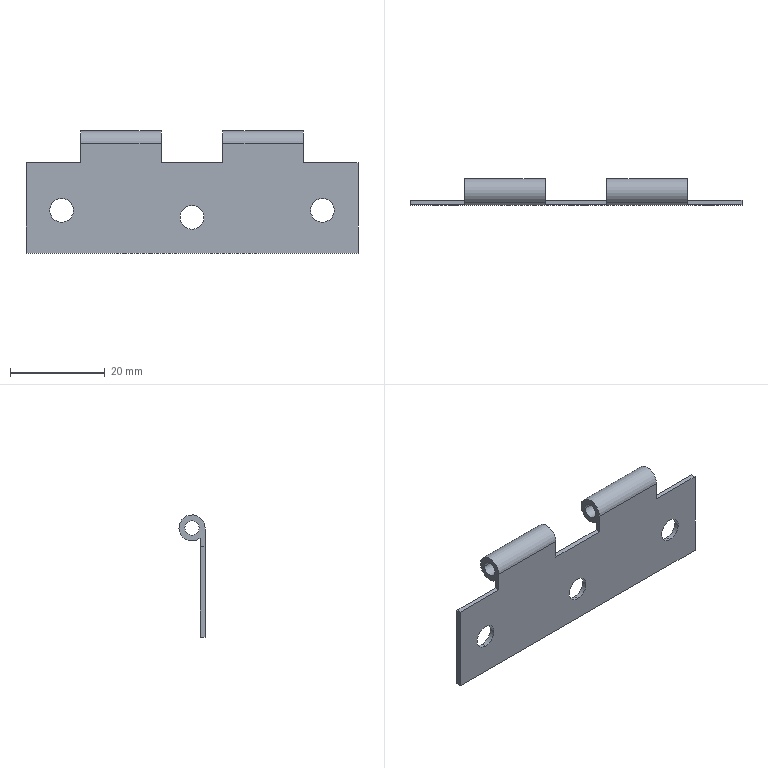Part | STEP file | 70 hinge-2 | 1 solid | 24 faces | box 70 x 5.5 x 25.75 mm | volume 1924 mm3 | cylinder 12 | plane 12 | commonest cylinder face diameters 5 x6 3 x4 5.5 x2